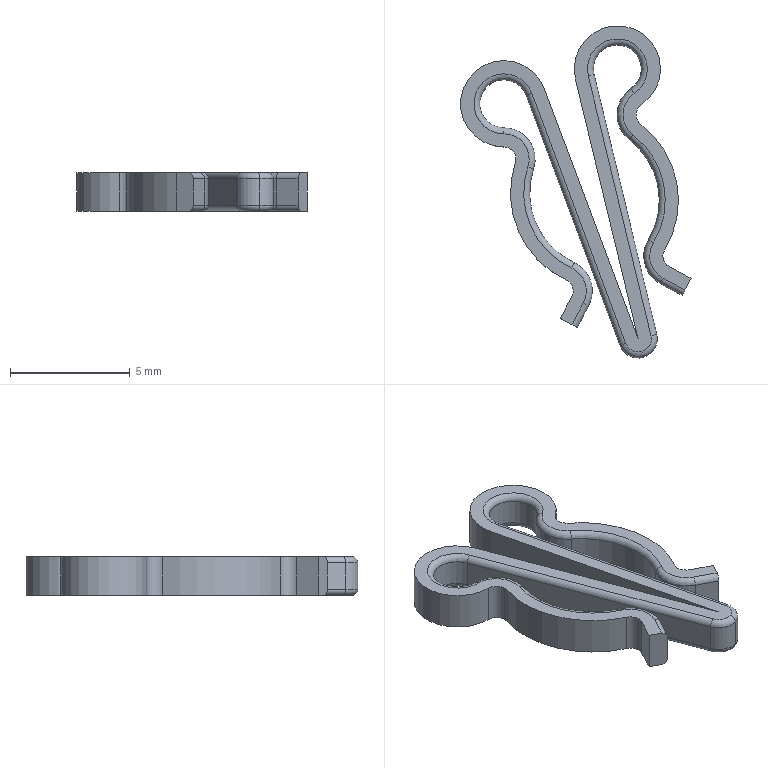Part | SolidWorks | features BaseBody 1 | 1 solid | 58 faces | box 9.607 x 13.853 x 1.6 mm | volume 68.431 mm3 | cylinder 26 | torus 20 | plane 12 | commonest cylinder face diameters 0.5 x8 1 x4 2.6 x4 1.6 x2 2 x2 3.6 x2